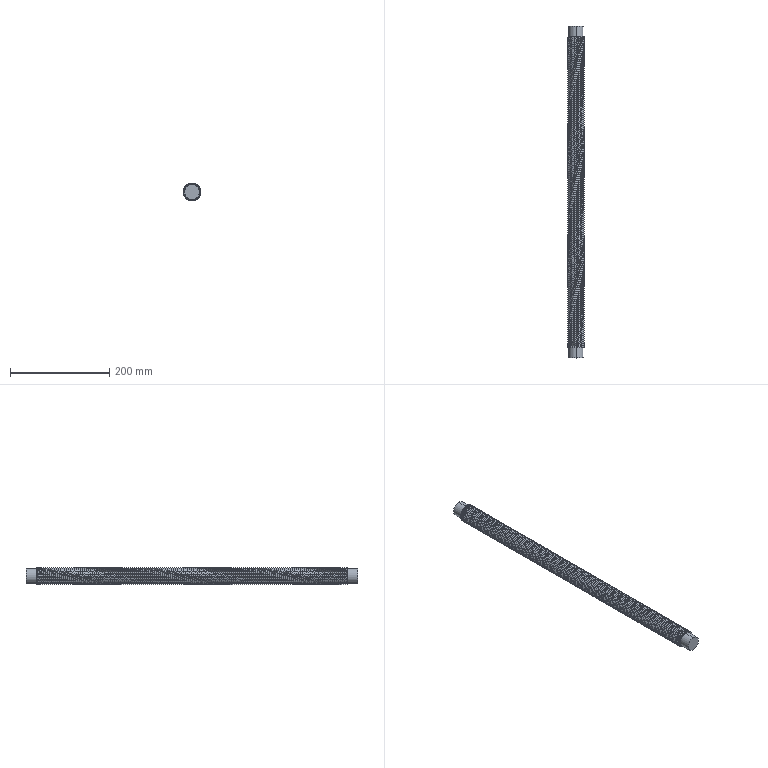Part | SolidWorks | features ICE 2, Extrusion 1, SweepThread 1 | 1 solid | 326 faces | box 36 x 670 x 36 mm | volume 568106 mm3 | cylinder 318 | plane 5 | spline 3 | commonest cylinder face diameters 36 x314 30 x4